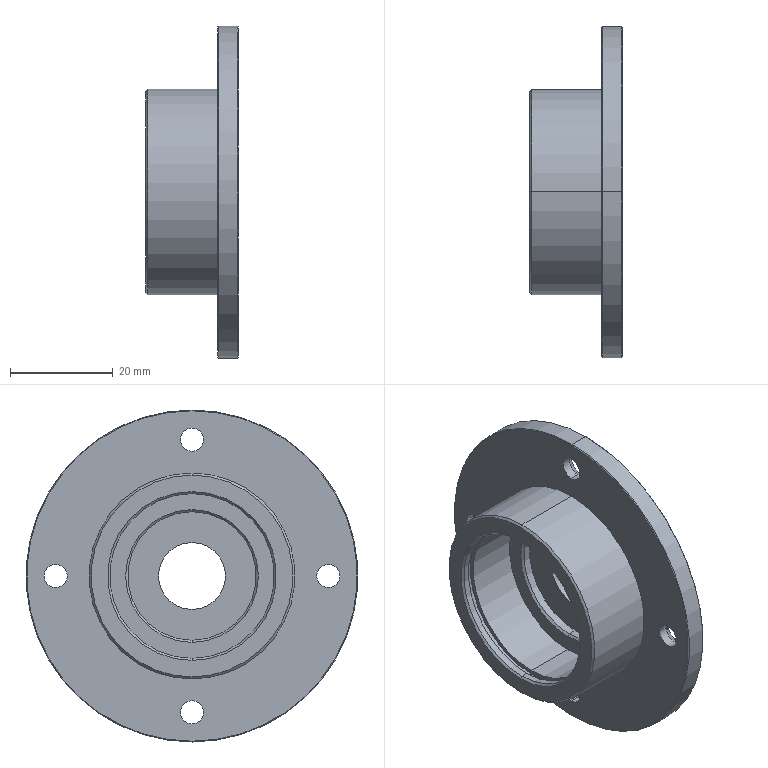Part | SolidWorks | features CirPattern 2, ICE 2, Chamfer 1, HoleWzd 1, RevCut 1, Revolution 1 | 1 solid | 47 faces | box 18 x 64.5 x 64.5 mm | volume 18239 mm3 | cylinder 22 | cone 18 | plane 7 | commonest cylinder face diameters 4.5 x8 32 x4 13 x2 25 x2 33.7 x2 40 x2
STEP:
#1=CARTESIAN_POINT('',(14.15,0.,32.25));
#2=VERTEX_POINT('',#1);
#3=CARTESIAN_POINT('',(14.15,0.,-32.25));
#4=VERTEX_POINT('',#3);
#5=CARTESIAN_POINT('',(14.15,0.,0.));
#6=DIRECTION('',(-1.,0.,0.));
#7=DIRECTION('',(0.,0.,-1.));
#8=AXIS2_PLACEMENT_3D('',#5,#6,#7);
#9=CIRCLE('',#8,32.25);
#10=EDGE_CURVE('',#2,#4,#9,.T.);
#11=ORIENTED_EDGE('',*,*,#10,.F.);
#12=CARTESIAN_POINT('',(17.85,0.,32.25));
#13=VERTEX_POINT('',#12);
#14=CARTESIAN_POINT('',(8.,0.,32.25));
#15=DIRECTION('',(1.,0.,0.));
#16=VECTOR('',#15,1000.);
#17=LINE('',#14,#16);
#18=EDGE_CURVE('',#2,#13,#17,.T.);
#19=ORIENTED_EDGE('',*,*,#18,.T.);
#20=CARTESIAN_POINT('',(17.85,0.,-32.25));
#21=VERTEX_POINT('',#20);
#22=CARTESIAN_POINT('',(17.85,0.,0.));
#23=DIRECTION('',(1.,0.,0.));
#24=DIRECTION('',(0.,0.,1.));
#25=AXIS2_PLACEMENT_3D('',#22,#23,#24);
#26=CIRCLE('',#25,32.25);
#27=EDGE_CURVE('',#21,#13,#26,.T.);
#28=ORIENTED_EDGE('',*,*,#27,.F.);
#29=CARTESIAN_POINT('',(8.,0.,-32.25));
#30=DIRECTION('',(1.,0.,0.));
#31=VECTOR('',#30,1000.);
#32=LINE('',#29,#31);
#33=EDGE_CURVE('',#4,#21,#32,.T.);
#34=ORIENTED_EDGE('',*,*,#33,.F.);
#35=EDGE_LOOP('',(#11,#19,#28,#34));
#36=FACE_OUTER_BOUND('',#35,.T.);
#37=CARTESIAN_POINT('',(8.,0.,0.));
#38=DIRECTION('',(1.,0.,0.));
#39=DIRECTION('',(0.,0.,-1.));
#40=AXIS2_PLACEMENT_3D('',#37,#38,#39);
#41=CYLINDRICAL_SURFACE('',#40,32.25);
#42=ADVANCED_FACE('',(#36),#41,.T.);
#43=CARTESIAN_POINT('',(18.,0.,-6.5));
#44=VERTEX_POINT('',#43);
#45=CARTESIAN_POINT('',(18.,0.,6.5));
#46=VERTEX_POINT('',#45);
#47=CARTESIAN_POINT('',(18.,0.,0.));
#48=DIRECTION('',(-1.,0.,0.));
#49=DIRECTION('',(0.,0.,1.));
#50=AXIS2_PLACEMENT_3D('',#47,#48,#49);
#51=CIRCLE('',#50,6.5);
#52=EDGE_CURVE('',#44,#46,#51,.T.);
#53=ORIENTED_EDGE('',*,*,#52,.F.);
#54=CARTESIAN_POINT('',(15.,0.,-6.5));
#55=VERTEX_POINT('',#54);
#56=CARTESIAN_POINT('',(25.,0.,-6.5));
#57=DIRECTION('',(-1.,0.,0.));
#58=VECTOR('',#57,1000.);
#59=LINE('',#56,#58);
#60=EDGE_CURVE('',#44,#55,#59,.T.);
#61=ORIENTED_EDGE('',*,*,#60,.T.);
#62=CARTESIAN_POINT('',(15.,0.,6.5));
#63=VERTEX_POINT('',#62);
#64=CARTESIAN_POINT('',(15.,0.,0.));
#65=DIRECTION('',(-1.,0.,0.));
#66=DIRECTION('',(0.,0.,1.));
#67=AXIS2_PLACEMENT_3D('',#64,#65,#66);
#68=CIRCLE('',#67,6.5);
#69=EDGE_CURVE('',#55,#63,#68,.T.);
#70=ORIENTED_EDGE('',*,*,#69,.T.);
#71=CARTESIAN_POINT('',(25.,0.,6.5));
#72=DIRECTION('',(-1.,0.,0.));
#73=VECTOR('',#72,1000.);
#74=LINE('',#71,#73);
#75=EDGE_CURVE('',#46,#63,#74,.T.);
#76=ORIENTED_EDGE('',*,*,#75,.F.);
#77=EDGE_LOOP('',(#53,#61,#70,#76));
#78=FACE_OUTER_BOUND('',#77,.T.);
#79=CARTESIAN_POINT('',(25.,0.,0.));
#80=DIRECTION('',(-1.,0.,0.));
#81=DIRECTION('',(0.,0.,1.));
#82=AXIS2_PLACEMENT_3D('',#79,#80,#81);
#83=CYLINDRICAL_SURFACE('',#82,6.5);
#84=ADVANCED_FACE('',(#78),#83,.F.);
#85=CARTESIAN_POINT('',(0.,0.,19.6));
#86=VERTEX_POINT('',#85);
#87=CARTESIAN_POINT('',(0.,0.,-19.6));
#88=VERTEX_POINT('',#87);
#89=CARTESIAN_POINT('',(0.,0.,0.));
#90=DIRECTION('',(-1.,0.,0.));
#91=DIRECTION('',(0.,0.,-1.));
#92=AXIS2_PLACEMENT_3D('',#89,#90,#91);
#93=CIRCLE('',#92,19.6);
#94=EDGE_CURVE('',#86,#88,#93,.T.);
#95=ORIENTED_EDGE('',*,*,#94,.F.);
#96=CARTESIAN_POINT('',(0.4,0.,20.));
#97=VERTEX_POINT('',#96);
#98=CARTESIAN_POINT('',(0.,0.,19.6));
#99=DIRECTION('',(0.7071,0.,0.7071));
#100=VECTOR('',#99,1000.);
#101=LINE('',#98,#100);
#102=EDGE_CURVE('',#86,#97,#101,.T.);
#103=ORIENTED_EDGE('',*,*,#102,.T.);
#104=CARTESIAN_POINT('',(0.4,0.,-20.));
#105=VERTEX_POINT('',#104);
#106=CARTESIAN_POINT('',(0.4,0.,0.));
#107=DIRECTION('',(1.,0.,0.));
#108=DIRECTION('',(0.,0.,-1.));
#109=AXIS2_PLACEMENT_3D('',#106,#107,#108);
#110=CIRCLE('',#109,20.);
#111=EDGE_CURVE('',#105,#97,#110,.T.);
#112=ORIENTED_EDGE('',*,*,#111,.F.);
#113=CARTESIAN_POINT('',(0.,0.,-19.6));
#114=DIRECTION('',(0.7071,0.,-0.7071));
#115=VECTOR('',#114,1000.);
#116=LINE('',#113,#115);
#117=EDGE_CURVE('',#88,#105,#116,.T.);
#118=ORIENTED_EDGE('',*,*,#117,.F.);
#119=EDGE_LOOP('',(#95,#103,#112,#118));
#120=FACE_OUTER_BOUND('',#119,.T.);
#121=CARTESIAN_POINT('',(0.,0.,0.));
#122=DIRECTION('',(1.,0.,0.));
#123=DIRECTION('',(0.,0.,-1.));
#124=AXIS2_PLACEMENT_3D('',#121,#122,#123);
#125=CONICAL_SURFACE('',#124,19.6,0.7854);
#126=ADVANCED_FACE('',(#120),#125,.T.);
#127=CARTESIAN_POINT('',(0.4,0.,-16.));
#128=VERTEX_POINT('',#127);
#129=CARTESIAN_POINT('',(0.4,0.,16.));
#130=VERTEX_POINT('',#129);
#131=CARTESIAN_POINT('',(0.4,0.,0.));
#132=DIRECTION('',(-1.,0.,0.));
#133=DIRECTION('',(0.,0.,-1.));
#134=AXIS2_PLACEMENT_3D('',#131,#132,#133);
#135=CIRCLE('',#134,16.);
#136=EDGE_CURVE('',#128,#130,#135,.T.);
#137=ORIENTED_EDGE('',*,*,#136,.F.);
#138=CARTESIAN_POINT('',(0.,0.,-16.4));
#139=VERTEX_POINT('',#138);
#140=CARTESIAN_POINT('',(0.4,0.,-16.));
#141=DIRECTION('',(-0.7071,0.,-0.7071));
#142=VECTOR('',#141,1000.);
#143=LINE('',#140,#142);
#144=EDGE_CURVE('',#128,#139,#143,.T.);
#145=ORIENTED_EDGE('',*,*,#144,.T.);
#146=CARTESIAN_POINT('',(0.,0.,16.4));
#147=VERTEX_POINT('',#146);
#148=CARTESIAN_POINT('',(0.,0.,0.));
#149=DIRECTION('',(1.,0.,0.));
#150=DIRECTION('',(0.,0.,-1.));
#151=AXIS2_PLACEMENT_3D('',#148,#149,#150);
#152=CIRCLE('',#151,16.4);
#153=EDGE_CURVE('',#147,#139,#152,.T.);
#154=ORIENTED_EDGE('',*,*,#153,.F.);
#155=CARTESIAN_POINT('',(0.4,0.,16.));
#156=DIRECTION('',(-0.7071,0.,0.7071));
#157=VECTOR('',#156,1000.);
#158=LINE('',#155,#157);
#159=EDGE_CURVE('',#130,#147,#158,.T.);
#160=ORIENTED_EDGE('',*,*,#159,.F.);
#161=EDGE_LOOP('',(#137,#145,#154,#160));
#162=FACE_OUTER_BOUND('',#161,.T.);
#163=CARTESIAN_POINT('',(0.4,0.,0.));
#164=DIRECTION('',(-1.,0.,0.));
#165=DIRECTION('',(0.,0.,1.));
#166=AXIS2_PLACEMENT_3D('',#163,#164,#165);
#167=CONICAL_SURFACE('',#166,16.,0.7854);
#168=ADVANCED_FACE('',(#162),#167,.F.);
#169=CARTESIAN_POINT('',(13.4,0.,-12.5));
#170=VERTEX_POINT('',#169);
#171=CARTESIAN_POINT('',(13.4,0.,12.5));
#172=VERTEX_POINT('',#171);
#173=CARTESIAN_POINT('',(13.4,0.,0.));
#174=DIRECTION('',(-1.,0.,0.));
#175=DIRECTION('',(0.,0.,-1.));
#176=AXIS2_PLACEMENT_3D('',#173,#174,#175);
#177=CIRCLE('',#176,12.5);
#178=EDGE_CURVE('',#170,#172,#177,.T.);
#179=ORIENTED_EDGE('',*,*,#178,.F.);
#180=CARTESIAN_POINT('',(13.,0.,-12.9));
#181=VERTEX_POINT('',#180);
#182=CARTESIAN_POINT('',(13.4,0.,-12.5));
#183=DIRECTION('',(-0.7071,0.,-0.7071));
#184=VECTOR('',#183,1000.);
#185=LINE('',#182,#184);
#186=EDGE_CURVE('',#170,#181,#185,.T.);
#187=ORIENTED_EDGE('',*,*,#186,.T.);
#188=CARTESIAN_POINT('',(13.,0.,12.9));
#189=VERTEX_POINT('',#188);
#190=CARTESIAN_POINT('',(13.,0.,0.));
#191=DIRECTION('',(1.,0.,0.));
#192=DIRECTION('',(0.,0.,-1.));
#193=AXIS2_PLACEMENT_3D('',#190,#191,#192);
#194=CIRCLE('',#193,12.9);
#195=EDGE_CURVE('',#189,#181,#194,.T.);
#196=ORIENTED_EDGE('',*,*,#195,.F.);
#197=CARTESIAN_POINT('',(13.4,0.,12.5));
#198=DIRECTION('',(-0.7071,0.,0.7071));
#199=VECTOR('',#198,1000.);
#200=LINE('',#197,#199);
#201=EDGE_CURVE('',#172,#189,#200,.T.);
#202=ORIENTED_EDGE('',*,*,#201,.F.);
#203=EDGE_LOOP('',(#179,#187,#196,#202));
#204=FACE_OUTER_BOUND('',#203,.T.);
#205=CARTESIAN_POINT('',(13.4,0.,0.));
#206=DIRECTION('',(-1.,0.,0.));
#207=DIRECTION('',(0.,0.,1.));
#208=AXIS2_PLACEMENT_3D('',#205,#206,#207);
#209=CONICAL_SURFACE('',#208,12.5,0.7854);
#210=ADVANCED_FACE('',(#204),#209,.F.);
#211=CARTESIAN_POINT('',(15.75,28.75,0.));
#212=VERTEX_POINT('',#211);
#213=CARTESIAN_POINT('',(15.75,24.25,0.));
#214=VERTEX_POINT('',#213);
#215=CARTESIAN_POINT('',(15.75,26.5,0.));
#216=DIRECTION('',(-1.,0.,0.));
#217=DIRECTION('',(0.,-1.,0.));
#218=AXIS2_PLACEMENT_3D('',#215,#216,#217);
#219=CIRCLE('',#218,2.25);
#220=EDGE_CURVE('',#212,#214,#219,.T.);
#221=ORIENTED_EDGE('',*,*,#220,.F.);
#222=CARTESIAN_POINT('',(14.,28.75,0.));
#223=VERTEX_POINT('',#222);
#224=CARTESIAN_POINT('',(14.,28.75,0.));
#225=DIRECTION('',(-1.,0.,0.));
#226=VECTOR('',#225,1000.);
#227=LINE('',#224,#226);
#228=EDGE_CURVE('',#212,#223,#227,.T.);
#229=ORIENTED_EDGE('',*,*,#228,.T.);
#230=CARTESIAN_POINT('',(14.,24.25,0.));
#231=VERTEX_POINT('',#230);
#232=CARTESIAN_POINT('',(14.,26.5,0.));
#233=DIRECTION('',(-1.,0.,0.));
#234=DIRECTION('',(0.,-1.,0.));
#235=AXIS2_PLACEMENT_3D('',#232,#233,#234);
#236=CIRCLE('',#235,2.25);
#237=EDGE_CURVE('',#223,#231,#236,.T.);
#238=ORIENTED_EDGE('',*,*,#237,.T.);
#239=CARTESIAN_POINT('',(14.,24.25,0.));
#240=DIRECTION('',(-1.,0.,0.));
#241=VECTOR('',#240,1000.);
#242=LINE('',#239,#241);
#243=EDGE_CURVE('',#214,#231,#242,.T.);
#244=ORIENTED_EDGE('',*,*,#243,.F.);
#245=EDGE_LOOP('',(#221,#229,#238,#244));
#246=FACE_OUTER_BOUND('',#245,.T.);
#247=CARTESIAN_POINT('',(14.,26.5,0.));
#248=DIRECTION('',(-1.,0.,0.));
#249=DIRECTION('',(0.,-1.,0.));
#250=AXIS2_PLACEMENT_3D('',#247,#248,#249);
#251=CYLINDRICAL_SURFACE('',#250,2.25);
#252=ADVANCED_FACE('',(#246),#251,.F.);
#253=ORIENTED_EDGE('',*,*,#220,.T.);
#254=CARTESIAN_POINT('',(18.,22.,0.));
#255=VERTEX_POINT('',#254);
#256=CARTESIAN_POINT('',(18.,22.,0.));
#257=DIRECTION('',(0.7071,-0.7071,0.));
#258=VECTOR('',#257,1000.);
#259=LINE('',#256,#258);
#260=EDGE_CURVE('',#214,#255,#259,.T.);
#261=ORIENTED_EDGE('',*,*,#260,.T.);
#262=CARTESIAN_POINT('',(18.,31.,0.));
#263=VERTEX_POINT('',#262);
#264=CARTESIAN_POINT('',(18.,26.5,0.));
#265=DIRECTION('',(-1.,0.,0.));
#266=DIRECTION('',(0.,-1.,0.));
#267=AXIS2_PLACEMENT_3D('',#264,#265,#266);
#268=CIRCLE('',#267,4.5);
#269=EDGE_CURVE('',#263,#255,#268,.T.);
#270=ORIENTED_EDGE('',*,*,#269,.F.);
#271=CARTESIAN_POINT('',(18.,31.,0.));
#272=DIRECTION('',(0.7071,0.7071,0.));
#273=VECTOR('',#272,1000.);
#274=LINE('',#271,#273);
#275=EDGE_CURVE('',#212,#263,#274,.T.);
#276=ORIENTED_EDGE('',*,*,#275,.F.);
#277=EDGE_LOOP('',(#253,#261,#270,#276));
#278=FACE_OUTER_BOUND('',#277,.T.);
#279=CARTESIAN_POINT('',(18.,26.5,0.));
#280=DIRECTION('',(1.,0.,0.));
#281=DIRECTION('',(0.,1.,0.));
#282=AXIS2_PLACEMENT_3D('',#279,#280,#281);
#283=CONICAL_SURFACE('',#282,4.5,0.7854);
#284=ADVANCED_FACE('',(#278),#283,.F.);
#285=CARTESIAN_POINT('',(15.75,0.,28.75));
#286=VERTEX_POINT('',#285);
#287=CARTESIAN_POINT('',(15.75,0.,24.25));
#288=VERTEX_POINT('',#287);
#289=CARTESIAN_POINT('',(15.75,0.,26.5));
#290=DIRECTION('',(-1.,0.,0.));
#291=DIRECTION('',(0.,0.,-1.));
#292=AXIS2_PLACEMENT_3D('',#289,#290,#291);
#293=CIRCLE('',#292,2.25);
#294=EDGE_CURVE('',#286,#288,#293,.T.);
#295=ORIENTED_EDGE('',*,*,#294,.F.);
#296=CARTESIAN_POINT('',(14.,0.,28.75));
#297=VERTEX_POINT('',#296);
#298=CARTESIAN_POINT('',(14.,0.,28.75));
#299=DIRECTION('',(-1.,0.,0.));
#300=VECTOR('',#299,1000.);
#301=LINE('',#298,#300);
#302=EDGE_CURVE('',#286,#297,#301,.T.);
#303=ORIENTED_EDGE('',*,*,#302,.T.);
#304=CARTESIAN_POINT('',(14.,0.,24.25));
#305=VERTEX_POINT('',#304);
#306=CARTESIAN_POINT('',(14.,0.,26.5));
#307=DIRECTION('',(-1.,0.,0.));
#308=DIRECTION('',(0.,0.,-1.));
#309=AXIS2_PLACEMENT_3D('',#306,#307,#308);
#310=CIRCLE('',#309,2.25);
#311=EDGE_CURVE('',#297,#305,#310,.T.);
#312=ORIENTED_EDGE('',*,*,#311,.T.);
#313=CARTESIAN_POINT('',(14.,0.,24.25));
#314=DIRECTION('',(-1.,0.,0.));
#315=VECTOR('',#314,1000.);
#316=LINE('',#313,#315);
#317=EDGE_CURVE('',#288,#305,#316,.T.);
#318=ORIENTED_EDGE('',*,*,#317,.F.);
#319=EDGE_LOOP('',(#295,#303,#312,#318));
#320=FACE_OUTER_BOUND('',#319,.T.);
#321=CARTESIAN_POINT('',(14.,0.,26.5));
#322=DIRECTION('',(-1.,0.,0.));
#323=DIRECTION('',(0.,0.,-1.));
#324=AXIS2_PLACEMENT_3D('',#321,#322,#323);
#325=CYLINDRICAL_SURFACE('',#324,2.25);
#326=ADVANCED_FACE('',(#320),#325,.F.);
#327=ORIENTED_EDGE('',*,*,#294,.T.);
#328=CARTESIAN_POINT('',(18.,0.,22.));
#329=VERTEX_POINT('',#328);
#330=CARTESIAN_POINT('',(18.,0.,22.));
#331=DIRECTION('',(0.7071,0.,-0.7071));
#332=VECTOR('',#331,1000.);
#333=LINE('',#330,#332);
#334=EDGE_CURVE('',#288,#329,#333,.T.);
#335=ORIENTED_EDGE('',*,*,#334,.T.);
#336=CARTESIAN_POINT('',(18.,0.,31.));
#337=VERTEX_POINT('',#336);
#338=CARTESIAN_POINT('',(18.,0.,26.5));
#339=DIRECTION('',(-1.,0.,0.));
#340=DIRECTION('',(0.,0.,-1.));
#341=AXIS2_PLACEMENT_3D('',#338,#339,#340);
#342=CIRCLE('',#341,4.5);
#343=EDGE_CURVE('',#337,#329,#342,.T.);
#344=ORIENTED_EDGE('',*,*,#343,.F.);
#345=CARTESIAN_POINT('',(18.,0.,31.));
#346=DIRECTION('',(0.7071,0.,0.7071));
#347=VECTOR('',#346,1000.);
#348=LINE('',#345,#347);
#349=EDGE_CURVE('',#286,#337,#348,.T.);
#350=ORIENTED_EDGE('',*,*,#349,.F.);
#351=EDGE_LOOP('',(#327,#335,#344,#350));
#352=FACE_OUTER_BOUND('',#351,.T.);
#353=CARTESIAN_POINT('',(18.,0.,26.5));
#354=DIRECTION('',(1.,0.,0.));
#355=DIRECTION('',(0.,0.,1.));
#356=AXIS2_PLACEMENT_3D('',#353,#354,#355);
#357=CONICAL_SURFACE('',#356,4.5,0.7854);
#358=ADVANCED_FACE('',(#352),#357,.F.);
#359=CARTESIAN_POINT('',(15.75,-28.75,0.));
#360=VERTEX_POINT('',#359);
#361=CARTESIAN_POINT('',(15.75,-24.25,0.));
#362=VERTEX_POINT('',#361);
#363=CARTESIAN_POINT('',(15.75,-26.5,0.));
#364=DIRECTION('',(-1.,0.,0.));
#365=DIRECTION('',(0.,1.,0.));
#366=AXIS2_PLACEMENT_3D('',#363,#364,#365);
#367=CIRCLE('',#366,2.25);
#368=EDGE_CURVE('',#360,#362,#367,.T.);
#369=ORIENTED_EDGE('',*,*,#368,.F.);
#370=CARTESIAN_POINT('',(14.,-28.75,0.));
#371=VERTEX_POINT('',#370);
#372=CARTESIAN_POINT('',(14.,-28.75,0.));
#373=DIRECTION('',(-1.,0.,0.));
#374=VECTOR('',#373,1000.);
#375=LINE('',#372,#374);
#376=EDGE_CURVE('',#360,#371,#375,.T.);
#377=ORIENTED_EDGE('',*,*,#376,.T.);
#378=CARTESIAN_POINT('',(14.,-24.25,0.));
#379=VERTEX_POINT('',#378);
#380=CARTESIAN_POINT('',(14.,-26.5,0.));
#381=DIRECTION('',(-1.,0.,0.));
#382=DIRECTION('',(0.,1.,0.));
#383=AXIS2_PLACEMENT_3D('',#380,#381,#382);
#384=CIRCLE('',#383,2.25);
#385=EDGE_CURVE('',#371,#379,#384,.T.);
#386=ORIENTED_EDGE('',*,*,#385,.T.);
#387=CARTESIAN_POINT('',(14.,-24.25,0.));
#388=DIRECTION('',(-1.,0.,0.));
#389=VECTOR('',#388,1000.);
#390=LINE('',#387,#389);
#391=EDGE_CURVE('',#362,#379,#390,.T.);
#392=ORIENTED_EDGE('',*,*,#391,.F.);
#393=EDGE_LOOP('',(#369,#377,#386,#392));
#394=FACE_OUTER_BOUND('',#393,.T.);
#395=CARTESIAN_POINT('',(14.,-26.5,0.));
#396=DIRECTION('',(-1.,0.,0.));
#397=DIRECTION('',(0.,1.,0.));
#398=AXIS2_PLACEMENT_3D('',#395,#396,#397);
#399=CYLINDRICAL_SURFACE('',#398,2.25);
#400=ADVANCED_FACE('',(#394),#399,.F.);
#401=ORIENTED_EDGE('',*,*,#368,.T.);
#402=CARTESIAN_POINT('',(18.,-22.,0.));
#403=VERTEX_POINT('',#402);
#404=CARTESIAN_POINT('',(18.,-22.,0.));
#405=DIRECTION('',(0.7071,0.7071,0.));
#406=VECTOR('',#405,1000.);
#407=LINE('',#404,#406);
#408=EDGE_CURVE('',#362,#403,#407,.T.);
#409=ORIENTED_EDGE('',*,*,#408,.T.);
#410=CARTESIAN_POINT('',(18.,-31.,0.));
#411=VERTEX_POINT('',#410);
#412=CARTESIAN_POINT('',(18.,-26.5,0.));
#413=DIRECTION('',(-1.,0.,0.));
#414=DIRECTION('',(0.,1.,0.));
#415=AXIS2_PLACEMENT_3D('',#412,#413,#414);
#416=CIRCLE('',#415,4.5);
#417=EDGE_CURVE('',#411,#403,#416,.T.);
#418=ORIENTED_EDGE('',*,*,#417,.F.);
#419=CARTESIAN_POINT('',(18.,-31.,0.));
#420=DIRECTION('',(0.7071,-0.7071,0.));
#421=VECTOR('',#420,1000.);
#422=LINE('',#419,#421);
#423=EDGE_CURVE('',#360,#411,#422,.T.);
#424=ORIENTED_EDGE('',*,*,#423,.F.);
#425=EDGE_LOOP('',(#401,#409,#418,#424));
#426=FACE_OUTER_BOUND('',#425,.T.);
#427=CARTESIAN_POINT('',(18.,-26.5,0.));
#428=DIRECTION('',(1.,0.,0.));
#429=DIRECTION('',(0.,-1.,0.));
#430=AXIS2_PLACEMENT_3D('',#427,#428,#429);
#431=CONICAL_SURFACE('',#430,4.5,0.7854);
#432=ADVANCED_FACE('',(#426),#431,.F.);
#433=CARTESIAN_POINT('',(15.75,0.,-28.75));
#434=VERTEX_POINT('',#433);
#435=CARTESIAN_POINT('',(15.75,0.,-24.25));
#436=VERTEX_POINT('',#435);
#437=CARTESIAN_POINT('',(15.75,0.,-26.5));
#438=DIRECTION('',(-1.,0.,0.));
#439=DIRECTION('',(0.,0.,1.));
#440=AXIS2_PLACEMENT_3D('',#437,#438,#439);
#441=CIRCLE('',#440,2.25);
#442=EDGE_CURVE('',#434,#436,#441,.T.);
#443=ORIENTED_EDGE('',*,*,#442,.F.);
#444=CARTESIAN_POINT('',(14.,0.,-28.75));
#445=VERTEX_POINT('',#444);
#446=CARTESIAN_POINT('',(14.,0.,-28.75));
#447=DIRECTION('',(-1.,0.,0.));
#448=VECTOR('',#447,1000.);
#449=LINE('',#446,#448);
#450=EDGE_CURVE('',#434,#445,#449,.T.);
#451=ORIENTED_EDGE('',*,*,#450,.T.);
#452=CARTESIAN_POINT('',(14.,0.,-24.25));
#453=VERTEX_POINT('',#452);
#454=CARTESIAN_POINT('',(14.,0.,-26.5));
#455=DIRECTION('',(-1.,0.,0.));
#456=DIRECTION('',(0.,0.,1.));
#457=AXIS2_PLACEMENT_3D('',#454,#455,#456);
#458=CIRCLE('',#457,2.25);
#459=EDGE_CURVE('',#445,#453,#458,.T.);
#460=ORIENTED_EDGE('',*,*,#459,.T.);
#461=CARTESIAN_POINT('',(14.,0.,-24.25));
#462=DIRECTION('',(-1.,0.,0.));
#463=VECTOR('',#462,1000.);
#464=LINE('',#461,#463);
#465=EDGE_CURVE('',#436,#453,#464,.T.);
#466=ORIENTED_EDGE('',*,*,#465,.F.);
#467=EDGE_LOOP('',(#443,#451,#460,#466));
#468=FACE_OUTER_BOUND('',#467,.T.);
#469=CARTESIAN_POINT('',(14.,0.,-26.5));
#470=DIRECTION('',(-1.,0.,0.));
#471=DIRECTION('',(0.,0.,1.));
#472=AXIS2_PLACEMENT_3D('',#469,#470,#471);
#473=CYLINDRICAL_SURFACE('',#472,2.25);
#474=ADVANCED_FACE('',(#468),#473,.F.);
#475=ORIENTED_EDGE('',*,*,#442,.T.);
#476=CARTESIAN_POINT('',(18.,0.,-22.));
#477=VERTEX_POINT('',#476);
#478=CARTESIAN_POINT('',(18.,0.,-22.));
#479=DIRECTION('',(0.7071,0.,0.7071));
#480=VECTOR('',#479,1000.);
#481=LINE('',#478,#480);
#482=EDGE_CURVE('',#436,#477,#481,.T.);
#483=ORIENTED_EDGE('',*,*,#482,.T.);
#484=CARTESIAN_POINT('',(18.,0.,-31.));
#485=VERTEX_POINT('',#484);
#486=CARTESIAN_POINT('',(18.,0.,-26.5));
#487=DIRECTION('',(-1.,0.,0.));
#488=DIRECTION('',(0.,0.,1.));
#489=AXIS2_PLACEMENT_3D('',#486,#487,#488);
#490=CIRCLE('',#489,4.5);
#491=EDGE_CURVE('',#485,#477,#490,.T.);
#492=ORIENTED_EDGE('',*,*,#491,.F.);
#493=CARTESIAN_POINT('',(18.,0.,-31.));
#494=DIRECTION('',(0.7071,0.,-0.7071));
#495=VECTOR('',#494,1000.);
#496=LINE('',#493,#495);
#497=EDGE_CURVE('',#434,#485,#496,.T.);
#498=ORIENTED_EDGE('',*,*,#497,.F.);
#499=EDGE_LOOP('',(#475,#483,#492,#498));
#500=FACE_OUTER_BOUND('',#499,.T.);
#501=CARTESIAN_POINT('',(18.,0.,-26.5));
#502=DIRECTION('',(1.,0.,0.));
#503=DIRECTION('',(0.,0.,-1.));
#504=AXIS2_PLACEMENT_3D('',#501,#502,#503);
#505=CONICAL_SURFACE('',#504,4.5,0.7854);
#506=ADVANCED_FACE('',(#500),#505,.F.);
#507=CARTESIAN_POINT('',(14.,0.,20.));
#508=VERTEX_POINT('',#507);
#509=CARTESIAN_POINT('',(14.,0.,-20.));
#510=VERTEX_POINT('',#509);
#511=CARTESIAN_POINT('',(14.,0.,0.));
#512=DIRECTION('',(-1.,0.,0.));
#513=DIRECTION('',(0.,0.,1.));
#514=AXIS2_PLACEMENT_3D('',#511,#512,#513);
#515=CIRCLE('',#514,20.);
#516=EDGE_CURVE('',#508,#510,#515,.T.);
#517=ORIENTED_EDGE('',*,*,#516,.T.);
#518=CARTESIAN_POINT('',(15.,0.,-20.));
#519=DIRECTION('',(-1.,0.,0.));
#520=VECTOR('',#519,1000.);
#521=LINE('',#518,#520);
#522=EDGE_CURVE('',#510,#105,#521,.T.);
#523=ORIENTED_EDGE('',*,*,#522,.T.);
#524=ORIENTED_EDGE('',*,*,#111,.T.);
#525=CARTESIAN_POINT('',(15.,0.,20.));
#526=DIRECTION('',(-1.,0.,0.));
#527=VECTOR('',#526,1000.);
#528=LINE('',#525,#527);
#529=EDGE_CURVE('',#508,#97,#528,.T.);
#530=ORIENTED_EDGE('',*,*,#529,.F.);
#531=EDGE_LOOP('',(#517,#523,#524,#530));
#532=FACE_OUTER_BOUND('',#531,.T.);
#533=CARTESIAN_POINT('',(15.,0.,0.));
#534=DIRECTION('',(-1.,0.,0.));
#535=DIRECTION('',(0.,0.,1.));
#536=AXIS2_PLACEMENT_3D('',#533,#534,#535);
#537=CYLINDRICAL_SURFACE('',#536,20.);
#538=ADVANCED_FACE('',(#532),#537,.T.);
#539=CARTESIAN_POINT('',(15.,0.,-12.5));
#540=VERTEX_POINT('',#539);
#541=CARTESIAN_POINT('',(15.,0.,12.5));
#542=VERTEX_POINT('',#541);
#543=CARTESIAN_POINT('',(15.,0.,0.));
#544=DIRECTION('',(-1.,0.,0.));
#545=DIRECTION('',(0.,0.,1.));
#546=AXIS2_PLACEMENT_3D('',#543,#544,#545);
#547=CIRCLE('',#546,12.5);
#548=EDGE_CURVE('',#540,#542,#547,.T.);
#549=ORIENTED_EDGE('',*,*,#548,.F.);
#550=CARTESIAN_POINT('',(15.,0.,-12.5));
#551=DIRECTION('',(-1.,0.,0.));
#552=VECTOR('',#551,1000.);
#553=LINE('',#550,#552);
#554=EDGE_CURVE('',#540,#170,#553,.T.);
#555=ORIENTED_EDGE('',*,*,#554,.T.);
#556=ORIENTED_EDGE('',*,*,#178,.T.);
#557=CARTESIAN_POINT('',(15.,0.,12.5));
#558=DIRECTION('',(-1.,0.,0.));
#559=VECTOR('',#558,1000.);
#560=LINE('',#557,#559);
#561=EDGE_CURVE('',#542,#172,#560,.T.);
#562=ORIENTED_EDGE('',*,*,#561,.F.);
#563=EDGE_LOOP('',(#549,#555,#556,#562));
#564=FACE_OUTER_BOUND('',#563,.T.);
#565=CARTESIAN_POINT('',(15.,0.,0.));
#566=DIRECTION('',(-1.,0.,0.));
#567=DIRECTION('',(0.,0.,1.));
#568=AXIS2_PLACEMENT_3D('',#565,#566,#567);
#569=CYLINDRICAL_SURFACE('',#568,12.5);
#570=ADVANCED_FACE('',(#564),#569,.F.);
#571=CARTESIAN_POINT('',(13.,0.,-16.));
#572=VERTEX_POINT('',#571);
#573=CARTESIAN_POINT('',(13.,0.,16.));
#574=VERTEX_POINT('',#573);
#575=CARTESIAN_POINT('',(13.,0.,0.));
#576=DIRECTION('',(-1.,0.,0.));
#577=DIRECTION('',(0.,0.,1.));
#578=AXIS2_PLACEMENT_3D('',#575,#576,#577);
#579=CIRCLE('',#578,16.);
#580=EDGE_CURVE('',#572,#574,#579,.T.);
#581=ORIENTED_EDGE('',*,*,#580,.F.);
#582=CARTESIAN_POINT('',(2.995,0.,-16.));
#583=VERTEX_POINT('',#582);
#584=CARTESIAN_POINT('',(15.,0.,-16.));
#585=DIRECTION('',(-1.,0.,0.));
#586=VECTOR('',#585,1000.);
#587=LINE('',#584,#586);
#588=EDGE_CURVE('',#572,#583,#587,.T.);
#589=ORIENTED_EDGE('',*,*,#588,.T.);
#590=CARTESIAN_POINT('',(2.995,0.,16.));
#591=VERTEX_POINT('',#590);
#592=CARTESIAN_POINT('',(2.995,0.,0.));
#593=DIRECTION('',(-1.,0.,0.));
#594=DIRECTION('',(0.,0.,1.));
#595=AXIS2_PLACEMENT_3D('',#592,#593,#594);
#596=CIRCLE('',#595,16.);
#597=EDGE_CURVE('',#583,#591,#596,.T.);
#598=ORIENTED_EDGE('',*,*,#597,.T.);
#599=CARTESIAN_POINT('',(15.,0.,16.));
#600=DIRECTION('',(-1.,0.,0.));
#601=VECTOR('',#600,1000.);
#602=LINE('',#599,#601);
#603=EDGE_CURVE('',#574,#591,#602,.T.);
#604=ORIENTED_EDGE('',*,*,#603,.F.);
#605=EDGE_LOOP('',(#581,#589,#598,#604));
#606=FACE_OUTER_BOUND('',#605,.T.);
#607=CARTESIAN_POINT('',(15.,0.,0.));
#608=DIRECTION('',(-1.,0.,0.));
#609=DIRECTION('',(0.,0.,1.));
#610=AXIS2_PLACEMENT_3D('',#607,#608,#609);
#611=CYLINDRICAL_SURFACE('',#610,16.);
#612=ADVANCED_FACE('',(#606),#611,.F.);
#613=CARTESIAN_POINT('',(2.995,0.,-16.85));
#614=VERTEX_POINT('',#613);
#615=CARTESIAN_POINT('',(2.995,0.,16.85));
#616=VERTEX_POINT('',#615);
#617=CARTESIAN_POINT('',(2.995,0.,0.));
#618=DIRECTION('',(-1.,0.,0.));
#619=DIRECTION('',(0.,0.,1.));
#620=AXIS2_PLACEMENT_3D('',#617,#618,#619);
#621=CIRCLE('',#620,16.85);
#622=EDGE_CURVE('',#614,#616,#621,.T.);
#623=ORIENTED_EDGE('',*,*,#622,.F.);
#624=CARTESIAN_POINT('',(1.695,0.,-16.85));
#625=VERTEX_POINT('',#624);
#626=CARTESIAN_POINT('',(15.,0.,-16.85));
#627=DIRECTION('',(-1.,0.,0.));
#628=VECTOR('',#627,1000.);
#629=LINE('',#626,#628);
#630=EDGE_CURVE('',#614,#625,#629,.T.);
#631=ORIENTED_EDGE('',*,*,#630,.T.);
#632=CARTESIAN_POINT('',(1.695,0.,16.85));
#633=VERTEX_POINT('',#632);
#634=CARTESIAN_POINT('',(1.695,0.,0.));
#635=DIRECTION('',(-1.,0.,0.));
#636=DIRECTION('',(0.,0.,1.));
#637=AXIS2_PLACEMENT_3D('',#634,#635,#636);
#638=CIRCLE('',#637,16.85);
#639=EDGE_CURVE('',#625,#633,#638,.T.);
#640=ORIENTED_EDGE('',*,*,#639,.T.);
#641=CARTESIAN_POINT('',(15.,0.,16.85));
#642=DIRECTION('',(-1.,0.,0.));
#643=VECTOR('',#642,1000.);
#644=LINE('',#641,#643);
#645=EDGE_CURVE('',#616,#633,#644,.T.);
#646=ORIENTED_EDGE('',*,*,#645,.F.);
#647=EDGE_LOOP('',(#623,#631,#640,#646));
#648=FACE_OUTER_BOUND('',#647,.T.);
#649=CARTESIAN_POINT('',(15.,0.,0.));
#650=DIRECTION('',(-1.,0.,0.));
#651=DIRECTION('',(0.,0.,1.));
#652=AXIS2_PLACEMENT_3D('',#649,#650,#651);
#653=CYLINDRICAL_SURFACE('',#652,16.85);
#654=ADVANCED_FACE('',(#648),#653,.F.);
#655=CARTESIAN_POINT('',(1.695,0.,-16.));
#656=VERTEX_POINT('',#655);
#657=CARTESIAN_POINT('',(1.695,0.,16.));
#658=VERTEX_POINT('',#657);
#659=CARTESIAN_POINT('',(1.695,0.,0.));
#660=DIRECTION('',(-1.,0.,0.));
#661=DIRECTION('',(0.,0.,1.));
#662=AXIS2_PLACEMENT_3D('',#659,#660,#661);
#663=CIRCLE('',#662,16.);
#664=EDGE_CURVE('',#656,#658,#663,.T.);
#665=ORIENTED_EDGE('',*,*,#664,.F.);
#666=CARTESIAN_POINT('',(15.,0.,-16.));
#667=DIRECTION('',(-1.,0.,0.));
#668=VECTOR('',#667,1000.);
#669=LINE('',#666,#668);
#670=EDGE_CURVE('',#656,#128,#669,.T.);
#671=ORIENTED_EDGE('',*,*,#670,.T.);
#672=ORIENTED_EDGE('',*,*,#136,.T.);
#673=CARTESIAN_POINT('',(15.,0.,16.));
#674=DIRECTION('',(-1.,0.,0.));
#675=VECTOR('',#674,1000.);
#676=LINE('',#673,#675);
#677=EDGE_CURVE('',#658,#130,#676,.T.);
#678=ORIENTED_EDGE('',*,*,#677,.F.);
#679=EDGE_LOOP('',(#665,#671,#672,#678));
#680=FACE_OUTER_BOUND('',#679,.T.);
#681=CARTESIAN_POINT('',(15.,0.,0.));
#682=DIRECTION('',(-1.,0.,0.));
#683=DIRECTION('',(0.,0.,1.));
#684=AXIS2_PLACEMENT_3D('',#681,#682,#683);
#685=CYLINDRICAL_SURFACE('',#684,16.);
#686=ADVANCED_FACE('',(#680),#685,.F.);
#687=CARTESIAN_POINT('',(14.,0.,32.1));
#688=VERTEX_POINT('',#687);
#689=CARTESIAN_POINT('',(14.,0.,-32.1));
#690=VERTEX_POINT('',#689);
#691=CARTESIAN_POINT('',(14.,0.,0.));
#692=DIRECTION('',(-1.,0.,0.));
#693=DIRECTION('',(0.,0.,-1.));
#694=AXIS2_PLACEMENT_3D('',#691,#692,#693);
#695=CIRCLE('',#694,32.1);
#696=EDGE_CURVE('',#688,#690,#695,.T.);
#697=ORIENTED_EDGE('',*,*,#696,.F.);
#698=CARTESIAN_POINT('',(14.,0.,32.1));
#699=DIRECTION('',(0.7071,0.,0.7071));
#700=VECTOR('',#699,1000.);
#701=LINE('',#698,#700);
#702=EDGE_CURVE('',#688,#2,#701,.T.);
#703=ORIENTED_EDGE('',*,*,#702,.T.);
#704=ORIENTED_EDGE('',*,*,#10,.T.);
#705=CARTESIAN_POINT('',(14.,0.,-32.1));
#706=DIRECTION('',(0.7071,0.,-0.7071));
#707=VECTOR('',#706,1000.);
#708=LINE('',#705,#707);
#709=EDGE_CURVE('',#690,#4,#708,.T.);
#710=ORIENTED_EDGE('',*,*,#709,.F.);
#711=EDGE_LOOP('',(#697,#703,#704,#710));
#712=FACE_OUTER_BOUND('',#711,.T.);
#713=CARTESIAN_POINT('',(14.,0.,0.));
#714=DIRECTION('',(1.,0.,0.));
#715=DIRECTION('',(0.,0.,-1.));
#716=AXIS2_PLACEMENT_3D('',#713,#714,#715);
#717=CONICAL_SURFACE('',#716,32.1,0.7854);
#718=ADVANCED_FACE('',(#712),#717,.T.);
#719=CARTESIAN_POINT('',(18.,0.,-32.1));
#720=VERTEX_POINT('',#719);
#721=CARTESIAN_POINT('',(18.,0.,32.1));
#722=VERTEX_POINT('',#721);
#723=CARTESIAN_POINT('',(18.,0.,0.));
#724=DIRECTION('',(1.,0.,0.));
#725=DIRECTION('',(0.,0.,1.));
#726=AXIS2_PLACEMENT_3D('',#723,#724,#725);
#727=CIRCLE('',#726,32.1);
#728=EDGE_CURVE('',#720,#722,#727,.T.);
#729=ORIENTED_EDGE('',*,*,#728,.F.);
#730=CARTESIAN_POINT('',(17.6,0.,-32.5));
#731=DIRECTION('',(-0.7071,0.,-0.7071));
#732=VECTOR('',#731,1000.);
#733=LINE('',#730,#732);
#734=EDGE_CURVE('',#720,#21,#733,.T.);
#735=ORIENTED_EDGE('',*,*,#734,.T.);
#736=ORIENTED_EDGE('',*,*,#27,.T.);
#737=CARTESIAN_POINT('',(17.6,0.,32.5));
#738=DIRECTION('',(-0.7071,0.,0.7071));
#739=VECTOR('',#738,1000.);
#740=LINE('',#737,#739);
#741=EDGE_CURVE('',#722,#13,#740,.T.);
#742=ORIENTED_EDGE('',*,*,#741,.F.);
#743=EDGE_LOOP('',(#729,#735,#736,#742));
#744=FACE_OUTER_BOUND('',#743,.T.);
#745=CARTESIAN_POINT('',(17.6,0.,0.));
#746=DIRECTION('',(-1.,0.,0.));
#747=DIRECTION('',(0.,0.,1.));
#748=AXIS2_PLACEMENT_3D('',#745,#746,#747);
#749=CONICAL_SURFACE('',#748,32.5,0.7854);
#750=ADVANCED_FACE('',(#744),#749,.T.);
#751=ORIENTED_EDGE('',*,*,#734,.F.);
#752=CARTESIAN_POINT('',(18.,0.,0.));
#753=DIRECTION('',(1.,0.,0.));
#754=DIRECTION('',(0.,0.,1.));
#755=AXIS2_PLACEMENT_3D('',#752,#753,#754);
#756=CIRCLE('',#755,32.1);
#757=EDGE_CURVE('',#722,#720,#756,.T.);
#758=ORIENTED_EDGE('',*,*,#757,.F.);
#759=ORIENTED_EDGE('',*,*,#741,.T.);
#760=CARTESIAN_POINT('',(17.85,0.,0.));
#761=DIRECTION('',(1.,0.,0.));
#762=DIRECTION('',(0.,0.,1.));
#763=AXIS2_PLACEMENT_3D('',#760,#761,#762);
#764=CIRCLE('',#763,32.25);
#765=EDGE_CURVE('',#13,#21,#764,.T.);
#766=ORIENTED_EDGE('',*,*,#765,.T.);
#767=EDGE_LOOP('',(#751,#758,#759,#766));
#768=FACE_OUTER_BOUND('',#767,.T.);
#769=CARTESIAN_POINT('',(17.6,0.,0.));
#770=DIRECTION('',(-1.,0.,0.));
#771=DIRECTION('',(0.,0.,1.));
#772=AXIS2_PLACEMENT_3D('',#769,#770,#771);
#773=CONICAL_SURFACE('',#772,32.5,0.7854);
#774=ADVANCED_FACE('',(#768),#773,.T.);
#775=ORIENTED_EDGE('',*,*,#702,.F.);
#776=CARTESIAN_POINT('',(14.,0.,0.));
#777=DIRECTION('',(-1.,0.,0.));
#778=DIRECTION('',(0.,0.,-1.));
#779=AXIS2_PLACEMENT_3D('',#776,#777,#778);
#780=CIRCLE('',#779,32.1);
#781=EDGE_CURVE('',#690,#688,#780,.T.);
#782=ORIENTED_EDGE('',*,*,#781,.F.);
#783=ORIENTED_EDGE('',*,*,#709,.T.);
#784=CARTESIAN_POINT('',(14.15,0.,0.));
#785=DIRECTION('',(-1.,0.,0.));
#786=DIRECTION('',(0.,0.,-1.));
#787=AXIS2_PLACEMENT_3D('',#784,#785,#786);
#788=CIRCLE('',#787,32.25);
#789=EDGE_CURVE('',#4,#2,#788,.T.);
#790=ORIENTED_EDGE('',*,*,#789,.T.);
#791=EDGE_LOOP('',(#775,#782,#783,#790));
#792=FACE_OUTER_BOUND('',#791,.T.);
#793=CARTESIAN_POINT('',(14.,0.,0.));
#794=DIRECTION('',(1.,0.,0.));
#795=DIRECTION('',(0.,0.,-1.));
#796=AXIS2_PLACEMENT_3D('',#793,#794,#795);
#797=CONICAL_SURFACE('',#796,32.1,0.7854);
#798=ADVANCED_FACE('',(#792),#797,.T.);
#799=ORIENTED_EDGE('',*,*,#153,.T.);
#800=CARTESIAN_POINT('',(0.,0.,0.));
#801=DIRECTION('',(1.,0.,0.));
#802=DIRECTION('',(0.,0.,-1.));
#803=AXIS2_PLACEMENT_3D('',#800,#801,#802);
#804=CIRCLE('',#803,16.4);
#805=EDGE_CURVE('',#139,#147,#804,.T.);
#806=ORIENTED_EDGE('',*,*,#805,.T.);
#807=EDGE_LOOP('',(#799,#806));
#808=FACE_BOUND('',#807,.T.);
#809=CARTESIAN_POINT('',(0.,0.,0.));
#810=DIRECTION('',(-1.,0.,0.));
#811=DIRECTION('',(0.,0.,-1.));
#812=AXIS2_PLACEMENT_3D('',#809,#810,#811);
#813=CIRCLE('',#812,19.6);
#814=EDGE_CURVE('',#88,#86,#813,.T.);
#815=ORIENTED_EDGE('',*,*,#814,.T.);
#816=ORIENTED_EDGE('',*,*,#94,.T.);
#817=EDGE_LOOP('',(#815,#816));
#818=FACE_OUTER_BOUND('',#817,.T.);
#819=CARTESIAN_POINT('',(0.,20.,0.));
#820=DIRECTION('',(1.,0.,0.));
#821=DIRECTION('',(0.,0.,-1.));
#822=AXIS2_PLACEMENT_3D('',#819,#820,#821);
#823=PLANE('',#822);
#824=ADVANCED_FACE('',(#808,#818),#823,.F.);
#825=ORIENTED_EDGE('',*,*,#670,.F.);
#826=CARTESIAN_POINT('',(1.695,0.,0.));
#827=DIRECTION('',(-1.,0.,0.));
#828=DIRECTION('',(0.,0.,1.));
#829=AXIS2_PLACEMENT_3D('',#826,#827,#828);
#830=CIRCLE('',#829,16.);
#831=EDGE_CURVE('',#658,#656,#830,.T.);
#832=ORIENTED_EDGE('',*,*,#831,.F.);
#833=ORIENTED_EDGE('',*,*,#677,.T.);
#834=CARTESIAN_POINT('',(0.4,0.,0.));
#835=DIRECTION('',(-1.,0.,0.));
#836=DIRECTION('',(0.,0.,-1.));
#837=AXIS2_PLACEMENT_3D('',#834,#835,#836);
#838=CIRCLE('',#837,16.);
#839=EDGE_CURVE('',#130,#128,#838,.T.);
#840=ORIENTED_EDGE('',*,*,#839,.T.);
#841=EDGE_LOOP('',(#825,#832,#833,#840));
#842=FACE_OUTER_BOUND('',#841,.T.);
#843=CARTESIAN_POINT('',(15.,0.,0.));
#844=DIRECTION('',(-1.,0.,0.));
#845=DIRECTION('',(0.,0.,1.));
#846=AXIS2_PLACEMENT_3D('',#843,#844,#845);
#847=CYLINDRICAL_SURFACE('',#846,16.);
#848=ADVANCED_FACE('',(#842),#847,.F.);
#849=CARTESIAN_POINT('',(1.695,0.,0.));
#850=DIRECTION('',(-1.,0.,0.));
#851=DIRECTION('',(0.,0.,1.));
#852=AXIS2_PLACEMENT_3D('',#849,#850,#851);
#853=CIRCLE('',#852,16.85);
#854=EDGE_CURVE('',#633,#625,#853,.T.);
#855=ORIENTED_EDGE('',*,*,#854,.F.);
#856=ORIENTED_EDGE('',*,*,#639,.F.);
#857=EDGE_LOOP('',(#855,#856));
#858=FACE_OUTER_BOUND('',#857,.T.);
#859=ORIENTED_EDGE('',*,*,#831,.T.);
#860=ORIENTED_EDGE('',*,*,#664,.T.);
#861=EDGE_LOOP('',(#859,#860));
#862=FACE_BOUND('',#861,.T.);
#863=CARTESIAN_POINT('',(1.695,16.,0.));
#864=DIRECTION('',(-1.,0.,0.));
#865=DIRECTION('',(0.,0.,1.));
#866=AXIS2_PLACEMENT_3D('',#863,#864,#865);
#867=PLANE('',#866);
#868=ADVANCED_FACE('',(#858,#862),#867,.F.);
#869=ORIENTED_EDGE('',*,*,#630,.F.);
#870=CARTESIAN_POINT('',(2.995,0.,0.));
#871=DIRECTION('',(-1.,0.,0.));
#872=DIRECTION('',(0.,0.,1.));
#873=AXIS2_PLACEMENT_3D('',#870,#871,#872);
#874=CIRCLE('',#873,16.85);
#875=EDGE_CURVE('',#616,#614,#874,.T.);
#876=ORIENTED_EDGE('',*,*,#875,.F.);
#877=ORIENTED_EDGE('',*,*,#645,.T.);
#878=ORIENTED_EDGE('',*,*,#854,.T.);
#879=EDGE_LOOP('',(#869,#876,#877,#878));
#880=FACE_OUTER_BOUND('',#879,.T.);
#881=CARTESIAN_POINT('',(15.,0.,0.));
#882=DIRECTION('',(-1.,0.,0.));
#883=DIRECTION('',(0.,0.,1.));
#884=AXIS2_PLACEMENT_3D('',#881,#882,#883);
#885=CYLINDRICAL_SURFACE('',#884,16.85);
#886=ADVANCED_FACE('',(#880),#885,.F.);
#887=CARTESIAN_POINT('',(2.995,0.,0.));
#888=DIRECTION('',(-1.,0.,0.));
#889=DIRECTION('',(0.,0.,1.));
#890=AXIS2_PLACEMENT_3D('',#887,#888,#889);
#891=CIRCLE('',#890,16.);
#892=EDGE_CURVE('',#591,#583,#891,.T.);
#893=ORIENTED_EDGE('',*,*,#892,.F.);
#894=ORIENTED_EDGE('',*,*,#597,.F.);
#895=EDGE_LOOP('',(#893,#894));
#896=FACE_BOUND('',#895,.T.);
#897=ORIENTED_EDGE('',*,*,#875,.T.);
#898=ORIENTED_EDGE('',*,*,#622,.T.);
#899=EDGE_LOOP('',(#897,#898));
#900=FACE_OUTER_BOUND('',#899,.T.);
#901=CARTESIAN_POINT('',(2.995,16.85,0.));
#902=DIRECTION('',(1.,0.,0.));
#903=DIRECTION('',(0.,0.,-1.));
#904=AXIS2_PLACEMENT_3D('',#901,#902,#903);
#905=PLANE('',#904);
#906=ADVANCED_FACE('',(#896,#900),#905,.F.);
#907=ORIENTED_EDGE('',*,*,#588,.F.);
#908=CARTESIAN_POINT('',(13.,0.,0.));
#909=DIRECTION('',(-1.,0.,0.));
#910=DIRECTION('',(0.,0.,1.));
#911=AXIS2_PLACEMENT_3D('',#908,#909,#910);
#912=CIRCLE('',#911,16.);
#913=EDGE_CURVE('',#574,#572,#912,.T.);
#914=ORIENTED_EDGE('',*,*,#913,.F.);
#915=ORIENTED_EDGE('',*,*,#603,.T.);
#916=ORIENTED_EDGE('',*,*,#892,.T.);
#917=EDGE_LOOP('',(#907,#914,#915,#916));
#918=FACE_OUTER_BOUND('',#917,.T.);
#919=CARTESIAN_POINT('',(15.,0.,0.));
#920=DIRECTION('',(-1.,0.,0.));
#921=DIRECTION('',(0.,0.,1.));
#922=AXIS2_PLACEMENT_3D('',#919,#920,#921);
#923=CYLINDRICAL_SURFACE('',#922,16.);
#924=ADVANCED_FACE('',(#918),#923,.F.);
#925=ORIENTED_EDGE('',*,*,#195,.T.);
#926=CARTESIAN_POINT('',(13.,0.,0.));
#927=DIRECTION('',(1.,0.,0.));
#928=DIRECTION('',(0.,0.,-1.));
#929=AXIS2_PLACEMENT_3D('',#926,#927,#928);
#930=CIRCLE('',#929,12.9);
#931=EDGE_CURVE('',#181,#189,#930,.T.);
#932=ORIENTED_EDGE('',*,*,#931,.T.);
#933=EDGE_LOOP('',(#925,#932));
#934=FACE_BOUND('',#933,.T.);
#935=ORIENTED_EDGE('',*,*,#913,.T.);
#936=ORIENTED_EDGE('',*,*,#580,.T.);
#937=EDGE_LOOP('',(#935,#936));
#938=FACE_OUTER_BOUND('',#937,.T.);
#939=CARTESIAN_POINT('',(13.,16.,0.));
#940=DIRECTION('',(1.,0.,0.));
#941=DIRECTION('',(0.,0.,-1.));
#942=AXIS2_PLACEMENT_3D('',#939,#940,#941);
#943=PLANE('',#942);
#944=ADVANCED_FACE('',(#934,#938),#943,.F.);
#945=ORIENTED_EDGE('',*,*,#554,.F.);
#946=CARTESIAN_POINT('',(15.,0.,0.));
#947=DIRECTION('',(-1.,0.,0.));
#948=DIRECTION('',(0.,0.,1.));
#949=AXIS2_PLACEMENT_3D('',#946,#947,#948);
#950=CIRCLE('',#949,12.5);
#951=EDGE_CURVE('',#542,#540,#950,.T.);
#952=ORIENTED_EDGE('',*,*,#951,.F.);
#953=ORIENTED_EDGE('',*,*,#561,.T.);
#954=CARTESIAN_POINT('',(13.4,0.,0.));
#955=DIRECTION('',(-1.,0.,0.));
#956=DIRECTION('',(0.,0.,-1.));
#957=AXIS2_PLACEMENT_3D('',#954,#955,#956);
#958=CIRCLE('',#957,12.5);
#959=EDGE_CURVE('',#172,#170,#958,.T.);
#960=ORIENTED_EDGE('',*,*,#959,.T.);
#961=EDGE_LOOP('',(#945,#952,#953,#960));
#962=FACE_OUTER_BOUND('',#961,.T.);
#963=CARTESIAN_POINT('',(15.,0.,0.));
#964=DIRECTION('',(-1.,0.,0.));
#965=DIRECTION('',(0.,0.,1.));
#966=AXIS2_PLACEMENT_3D('',#963,#964,#965);
#967=CYLINDRICAL_SURFACE('',#966,12.5);
#968=ADVANCED_FACE('',(#962),#967,.F.);
#969=CARTESIAN_POINT('',(15.,0.,0.));
#970=DIRECTION('',(-1.,0.,0.));
#971=DIRECTION('',(0.,0.,1.));
#972=AXIS2_PLACEMENT_3D('',#969,#970,#971);
#973=CIRCLE('',#972,6.5);
#974=EDGE_CURVE('',#63,#55,#973,.T.);
#975=ORIENTED_EDGE('',*,*,#974,.F.);
#976=ORIENTED_EDGE('',*,*,#69,.F.);
#977=EDGE_LOOP('',(#975,#976));
#978=FACE_BOUND('',#977,.T.);
#979=ORIENTED_EDGE('',*,*,#951,.T.);
#980=ORIENTED_EDGE('',*,*,#548,.T.);
#981=EDGE_LOOP('',(#979,#980));
#982=FACE_OUTER_BOUND('',#981,.T.);
#983=CARTESIAN_POINT('',(15.,12.5,0.));
#984=DIRECTION('',(1.,0.,0.));
#985=DIRECTION('',(0.,0.,-1.));
#986=AXIS2_PLACEMENT_3D('',#983,#984,#985);
#987=PLANE('',#986);
#988=ADVANCED_FACE('',(#978,#982),#987,.F.);
#989=CARTESIAN_POINT('',(18.,0.,0.));
#990=DIRECTION('',(-1.,0.,0.));
#991=DIRECTION('',(0.,0.,1.));
#992=AXIS2_PLACEMENT_3D('',#989,#990,#991);
#993=CIRCLE('',#992,6.5);
#994=EDGE_CURVE('',#46,#44,#993,.T.);
#995=ORIENTED_EDGE('',*,*,#994,.T.);
#996=ORIENTED_EDGE('',*,*,#52,.T.);
#997=EDGE_LOOP('',(#995,#996));
#998=FACE_BOUND('',#997,.T.);
#999=ORIENTED_EDGE('',*,*,#757,.T.);
#1000=ORIENTED_EDGE('',*,*,#728,.T.);
#1001=EDGE_LOOP('',(#999,#1000));
#1002=FACE_OUTER_BOUND('',#1001,.T.);
#1003=ORIENTED_EDGE('',*,*,#269,.T.);
#1004=CARTESIAN_POINT('',(18.,26.5,0.));
#1005=DIRECTION('',(-1.,0.,0.));
#1006=DIRECTION('',(0.,-1.,0.));
#1007=AXIS2_PLACEMENT_3D('',#1004,#1005,#1006);
#1008=CIRCLE('',#1007,4.5);
#1009=EDGE_CURVE('',#255,#263,#1008,.T.);
#1010=ORIENTED_EDGE('',*,*,#1009,.T.);
#1011=EDGE_LOOP('',(#1003,#1010));
#1012=FACE_BOUND('',#1011,.T.);
#1013=ORIENTED_EDGE('',*,*,#343,.T.);
#1014=CARTESIAN_POINT('',(18.,0.,26.5));
#1015=DIRECTION('',(-1.,0.,0.));
#1016=DIRECTION('',(0.,0.,-1.));
#1017=AXIS2_PLACEMENT_3D('',#1014,#1015,#1016);
#1018=CIRCLE('',#1017,4.5);
#1019=EDGE_CURVE('',#329,#337,#1018,.T.);
#1020=ORIENTED_EDGE('',*,*,#1019,.T.);
#1021=EDGE_LOOP('',(#1013,#1020));
#1022=FACE_BOUND('',#1021,.T.);
#1023=ORIENTED_EDGE('',*,*,#417,.T.);
#1024=CARTESIAN_POINT('',(18.,-26.5,0.));
#1025=DIRECTION('',(-1.,0.,0.));
#1026=DIRECTION('',(0.,1.,0.));
#1027=AXIS2_PLACEMENT_3D('',#1024,#1025,#1026);
#1028=CIRCLE('',#1027,4.5);
#1029=EDGE_CURVE('',#403,#411,#1028,.T.);
#1030=ORIENTED_EDGE('',*,*,#1029,.T.);
#1031=EDGE_LOOP('',(#1023,#1030));
#1032=FACE_BOUND('',#1031,.T.);
#1033=ORIENTED_EDGE('',*,*,#491,.T.);
#1034=CARTESIAN_POINT('',(18.,0.,-26.5));
#1035=DIRECTION('',(-1.,0.,0.));
#1036=DIRECTION('',(0.,0.,1.));
#1037=AXIS2_PLACEMENT_3D('',#1034,#1035,#1036);
#1038=CIRCLE('',#1037,4.5);
#1039=EDGE_CURVE('',#477,#485,#1038,.T.);
#1040=ORIENTED_EDGE('',*,*,#1039,.T.);
#1041=EDGE_LOOP('',(#1033,#1040));
#1042=FACE_BOUND('',#1041,.T.);
#1043=CARTESIAN_POINT('',(18.,0.,0.));
#1044=DIRECTION('',(-1.,0.,0.));
#1045=DIRECTION('',(0.,0.,1.));
#1046=AXIS2_PLACEMENT_3D('',#1043,#1044,#1045);
#1047=PLANE('',#1046);
#1048=ADVANCED_FACE('',(#998,#1002,#1012,#1022,#1032,#1042),#1047,.F.);
#1049=ORIENTED_EDGE('',*,*,#781,.T.);
#1050=ORIENTED_EDGE('',*,*,#696,.T.);
#1051=EDGE_LOOP('',(#1049,#1050));
#1052=FACE_OUTER_BOUND('',#1051,.T.);
#1053=CARTESIAN_POINT('',(14.,26.5,0.));
#1054=DIRECTION('',(-1.,0.,0.));
#1055=DIRECTION('',(0.,-1.,0.));
#1056=AXIS2_PLACEMENT_3D('',#1053,#1054,#1055);
#1057=CIRCLE('',#1056,2.25);
#1058=EDGE_CURVE('',#231,#223,#1057,.T.);
#1059=ORIENTED_EDGE('',*,*,#1058,.F.);
#1060=ORIENTED_EDGE('',*,*,#237,.F.);
#1061=EDGE_LOOP('',(#1059,#1060));
#1062=FACE_BOUND('',#1061,.T.);
#1063=CARTESIAN_POINT('',(14.,0.,26.5));
#1064=DIRECTION('',(-1.,0.,0.));
#1065=DIRECTION('',(0.,0.,-1.));
#1066=AXIS2_PLACEMENT_3D('',#1063,#1064,#1065);
#1067=CIRCLE('',#1066,2.25);
#1068=EDGE_CURVE('',#305,#297,#1067,.T.);
#1069=ORIENTED_EDGE('',*,*,#1068,.F.);
#1070=ORIENTED_EDGE('',*,*,#311,.F.);
#1071=EDGE_LOOP('',(#1069,#1070));
#1072=FACE_BOUND('',#1071,.T.);
#1073=CARTESIAN_POINT('',(14.,-26.5,0.));
#1074=DIRECTION('',(-1.,0.,0.));
#1075=DIRECTION('',(0.,1.,0.));
#1076=AXIS2_PLACEMENT_3D('',#1073,#1074,#1075);
#1077=CIRCLE('',#1076,2.25);
#1078=EDGE_CURVE('',#379,#371,#1077,.T.);
#1079=ORIENTED_EDGE('',*,*,#1078,.F.);
#1080=ORIENTED_EDGE('',*,*,#385,.F.);
#1081=EDGE_LOOP('',(#1079,#1080));
#1082=FACE_BOUND('',#1081,.T.);
#1083=CARTESIAN_POINT('',(14.,0.,-26.5));
#1084=DIRECTION('',(-1.,0.,0.));
#1085=DIRECTION('',(0.,0.,1.));
#1086=AXIS2_PLACEMENT_3D('',#1083,#1084,#1085);
#1087=CIRCLE('',#1086,2.25);
#1088=EDGE_CURVE('',#453,#445,#1087,.T.);
#1089=ORIENTED_EDGE('',*,*,#1088,.F.);
#1090=ORIENTED_EDGE('',*,*,#459,.F.);
#1091=EDGE_LOOP('',(#1089,#1090));
#1092=FACE_BOUND('',#1091,.T.);
#1093=ORIENTED_EDGE('',*,*,#516,.F.);
#1094=CARTESIAN_POINT('',(14.,0.,0.));
#1095=DIRECTION('',(-1.,0.,0.));
#1096=DIRECTION('',(0.,0.,1.));
#1097=AXIS2_PLACEMENT_3D('',#1094,#1095,#1096);
#1098=CIRCLE('',#1097,20.);
#1099=EDGE_CURVE('',#510,#508,#1098,.T.);
#1100=ORIENTED_EDGE('',*,*,#1099,.F.);
#1101=EDGE_LOOP('',(#1093,#1100));
#1102=FACE_BOUND('',#1101,.T.);
#1103=CARTESIAN_POINT('',(14.,32.5,0.));
#1104=DIRECTION('',(1.,0.,0.));
#1105=DIRECTION('',(0.,0.,-1.));
#1106=AXIS2_PLACEMENT_3D('',#1103,#1104,#1105);
#1107=PLANE('',#1106);
#1108=ADVANCED_FACE('',(#1052,#1062,#1072,#1082,#1092,#1102),#1107,.F.);
#1109=ORIENTED_EDGE('',*,*,#522,.F.);
#1110=ORIENTED_EDGE('',*,*,#1099,.T.);
#1111=ORIENTED_EDGE('',*,*,#529,.T.);
#1112=CARTESIAN_POINT('',(0.4,0.,0.));
#1113=DIRECTION('',(1.,0.,0.));
#1114=DIRECTION('',(0.,0.,-1.));
#1115=AXIS2_PLACEMENT_3D('',#1112,#1113,#1114);
#1116=CIRCLE('',#1115,20.);
#1117=EDGE_CURVE('',#97,#105,#1116,.T.);
#1118=ORIENTED_EDGE('',*,*,#1117,.T.);
#1119=EDGE_LOOP('',(#1109,#1110,#1111,#1118));
#1120=FACE_OUTER_BOUND('',#1119,.T.);
#1121=CARTESIAN_POINT('',(15.,0.,0.));
#1122=DIRECTION('',(-1.,0.,0.));
#1123=DIRECTION('',(0.,0.,1.));
#1124=AXIS2_PLACEMENT_3D('',#1121,#1122,#1123);
#1125=CYLINDRICAL_SURFACE('',#1124,20.);
#1126=ADVANCED_FACE('',(#1120),#1125,.T.);
#1127=ORIENTED_EDGE('',*,*,#482,.F.);
#1128=CARTESIAN_POINT('',(15.75,0.,-26.5));
#1129=DIRECTION('',(-1.,0.,0.));
#1130=DIRECTION('',(0.,0.,1.));
#1131=AXIS2_PLACEMENT_3D('',#1128,#1129,#1130);
#1132=CIRCLE('',#1131,2.25);
#1133=EDGE_CURVE('',#436,#434,#1132,.T.);
#1134=ORIENTED_EDGE('',*,*,#1133,.T.);
#1135=ORIENTED_EDGE('',*,*,#497,.T.);
#1136=ORIENTED_EDGE('',*,*,#1039,.F.);
#1137=EDGE_LOOP('',(#1127,#1134,#1135,#1136));
#1138=FACE_OUTER_BOUND('',#1137,.T.);
#1139=CARTESIAN_POINT('',(18.,0.,-26.5));
#1140=DIRECTION('',(1.,0.,0.));
#1141=DIRECTION('',(0.,0.,-1.));
#1142=AXIS2_PLACEMENT_3D('',#1139,#1140,#1141);
#1143=CONICAL_SURFACE('',#1142,4.5,0.7854);
#1144=ADVANCED_FACE('',(#1138),#1143,.F.);
#1145=ORIENTED_EDGE('',*,*,#450,.F.);
#1146=ORIENTED_EDGE('',*,*,#1133,.F.);
#1147=ORIENTED_EDGE('',*,*,#465,.T.);
#1148=ORIENTED_EDGE('',*,*,#1088,.T.);
#1149=EDGE_LOOP('',(#1145,#1146,#1147,#1148));
#1150=FACE_OUTER_BOUND('',#1149,.T.);
#1151=CARTESIAN_POINT('',(14.,0.,-26.5));
#1152=DIRECTION('',(-1.,0.,0.));
#1153=DIRECTION('',(0.,0.,1.));
#1154=AXIS2_PLACEMENT_3D('',#1151,#1152,#1153);
#1155=CYLINDRICAL_SURFACE('',#1154,2.25);
#1156=ADVANCED_FACE('',(#1150),#1155,.F.);
#1157=ORIENTED_EDGE('',*,*,#408,.F.);
#1158=CARTESIAN_POINT('',(15.75,-26.5,0.));
#1159=DIRECTION('',(-1.,0.,0.));
#1160=DIRECTION('',(0.,1.,0.));
#1161=AXIS2_PLACEMENT_3D('',#1158,#1159,#1160);
#1162=CIRCLE('',#1161,2.25);
#1163=EDGE_CURVE('',#362,#360,#1162,.T.);
#1164=ORIENTED_EDGE('',*,*,#1163,.T.);
#1165=ORIENTED_EDGE('',*,*,#423,.T.);
#1166=ORIENTED_EDGE('',*,*,#1029,.F.);
#1167=EDGE_LOOP('',(#1157,#1164,#1165,#1166));
#1168=FACE_OUTER_BOUND('',#1167,.T.);
#1169=CARTESIAN_POINT('',(18.,-26.5,0.));
#1170=DIRECTION('',(1.,0.,0.));
#1171=DIRECTION('',(0.,-1.,0.));
#1172=AXIS2_PLACEMENT_3D('',#1169,#1170,#1171);
#1173=CONICAL_SURFACE('',#1172,4.5,0.7854);
#1174=ADVANCED_FACE('',(#1168),#1173,.F.);
#1175=ORIENTED_EDGE('',*,*,#376,.F.);
#1176=ORIENTED_EDGE('',*,*,#1163,.F.);
#1177=ORIENTED_EDGE('',*,*,#391,.T.);
#1178=ORIENTED_EDGE('',*,*,#1078,.T.);
#1179=EDGE_LOOP('',(#1175,#1176,#1177,#1178));
#1180=FACE_OUTER_BOUND('',#1179,.T.);
#1181=CARTESIAN_POINT('',(14.,-26.5,0.));
#1182=DIRECTION('',(-1.,0.,0.));
#1183=DIRECTION('',(0.,1.,0.));
#1184=AXIS2_PLACEMENT_3D('',#1181,#1182,#1183);
#1185=CYLINDRICAL_SURFACE('',#1184,2.25);
#1186=ADVANCED_FACE('',(#1180),#1185,.F.);
#1187=ORIENTED_EDGE('',*,*,#334,.F.);
#1188=CARTESIAN_POINT('',(15.75,0.,26.5));
#1189=DIRECTION('',(-1.,0.,0.));
#1190=DIRECTION('',(0.,0.,-1.));
#1191=AXIS2_PLACEMENT_3D('',#1188,#1189,#1190);
#1192=CIRCLE('',#1191,2.25);
#1193=EDGE_CURVE('',#288,#286,#1192,.T.);
#1194=ORIENTED_EDGE('',*,*,#1193,.T.);
#1195=ORIENTED_EDGE('',*,*,#349,.T.);
#1196=ORIENTED_EDGE('',*,*,#1019,.F.);
#1197=EDGE_LOOP('',(#1187,#1194,#1195,#1196));
#1198=FACE_OUTER_BOUND('',#1197,.T.);
#1199=CARTESIAN_POINT('',(18.,0.,26.5));
#1200=DIRECTION('',(1.,0.,0.));
#1201=DIRECTION('',(0.,0.,1.));
#1202=AXIS2_PLACEMENT_3D('',#1199,#1200,#1201);
#1203=CONICAL_SURFACE('',#1202,4.5,0.7854);
#1204=ADVANCED_FACE('',(#1198),#1203,.F.);
#1205=ORIENTED_EDGE('',*,*,#302,.F.);
#1206=ORIENTED_EDGE('',*,*,#1193,.F.);
#1207=ORIENTED_EDGE('',*,*,#317,.T.);
#1208=ORIENTED_EDGE('',*,*,#1068,.T.);
#1209=EDGE_LOOP('',(#1205,#1206,#1207,#1208));
#1210=FACE_OUTER_BOUND('',#1209,.T.);
#1211=CARTESIAN_POINT('',(14.,0.,26.5));
#1212=DIRECTION('',(-1.,0.,0.));
#1213=DIRECTION('',(0.,0.,-1.));
#1214=AXIS2_PLACEMENT_3D('',#1211,#1212,#1213);
#1215=CYLINDRICAL_SURFACE('',#1214,2.25);
#1216=ADVANCED_FACE('',(#1210),#1215,.F.);
#1217=ORIENTED_EDGE('',*,*,#260,.F.);
#1218=CARTESIAN_POINT('',(15.75,26.5,0.));
#1219=DIRECTION('',(-1.,0.,0.));
#1220=DIRECTION('',(0.,-1.,0.));
#1221=AXIS2_PLACEMENT_3D('',#1218,#1219,#1220);
#1222=CIRCLE('',#1221,2.25);
#1223=EDGE_CURVE('',#214,#212,#1222,.T.);
#1224=ORIENTED_EDGE('',*,*,#1223,.T.);
#1225=ORIENTED_EDGE('',*,*,#275,.T.);
#1226=ORIENTED_EDGE('',*,*,#1009,.F.);
#1227=EDGE_LOOP('',(#1217,#1224,#1225,#1226));
#1228=FACE_OUTER_BOUND('',#1227,.T.);
#1229=CARTESIAN_POINT('',(18.,26.5,0.));
#1230=DIRECTION('',(1.,0.,0.));
#1231=DIRECTION('',(0.,1.,0.));
#1232=AXIS2_PLACEMENT_3D('',#1229,#1230,#1231);
#1233=CONICAL_SURFACE('',#1232,4.5,0.7854);
#1234=ADVANCED_FACE('',(#1228),#1233,.F.);
#1235=ORIENTED_EDGE('',*,*,#228,.F.);
#1236=ORIENTED_EDGE('',*,*,#1223,.F.);
#1237=ORIENTED_EDGE('',*,*,#243,.T.);
#1238=ORIENTED_EDGE('',*,*,#1058,.T.);
#1239=EDGE_LOOP('',(#1235,#1236,#1237,#1238));
#1240=FACE_OUTER_BOUND('',#1239,.T.);
#1241=CARTESIAN_POINT('',(14.,26.5,0.));
#1242=DIRECTION('',(-1.,0.,0.));
#1243=DIRECTION('',(0.,-1.,0.));
#1244=AXIS2_PLACEMENT_3D('',#1241,#1242,#1243);
#1245=CYLINDRICAL_SURFACE('',#1244,2.25);
#1246=ADVANCED_FACE('',(#1240),#1245,.F.);
#1247=ORIENTED_EDGE('',*,*,#186,.F.);
#1248=ORIENTED_EDGE('',*,*,#959,.F.);
#1249=ORIENTED_EDGE('',*,*,#201,.T.);
#1250=ORIENTED_EDGE('',*,*,#931,.F.);
#1251=EDGE_LOOP('',(#1247,#1248,#1249,#1250));
#1252=FACE_OUTER_BOUND('',#1251,.T.);
#1253=CARTESIAN_POINT('',(13.4,0.,0.));
#1254=DIRECTION('',(-1.,0.,0.));
#1255=DIRECTION('',(0.,0.,1.));
#1256=AXIS2_PLACEMENT_3D('',#1253,#1254,#1255);
#1257=CONICAL_SURFACE('',#1256,12.5,0.7854);
#1258=ADVANCED_FACE('',(#1252),#1257,.F.);
#1259=ORIENTED_EDGE('',*,*,#144,.F.);
#1260=ORIENTED_EDGE('',*,*,#839,.F.);
#1261=ORIENTED_EDGE('',*,*,#159,.T.);
#1262=ORIENTED_EDGE('',*,*,#805,.F.);
#1263=EDGE_LOOP('',(#1259,#1260,#1261,#1262));
#1264=FACE_OUTER_BOUND('',#1263,.T.);
#1265=CARTESIAN_POINT('',(0.4,0.,0.));
#1266=DIRECTION('',(-1.,0.,0.));
#1267=DIRECTION('',(0.,0.,1.));
#1268=AXIS2_PLACEMENT_3D('',#1265,#1266,#1267);
#1269=CONICAL_SURFACE('',#1268,16.,0.7854);
#1270=ADVANCED_FACE('',(#1264),#1269,.F.);
#1271=ORIENTED_EDGE('',*,*,#102,.F.);
#1272=ORIENTED_EDGE('',*,*,#814,.F.);
#1273=ORIENTED_EDGE('',*,*,#117,.T.);
#1274=ORIENTED_EDGE('',*,*,#1117,.F.);
#1275=EDGE_LOOP('',(#1271,#1272,#1273,#1274));
#1276=FACE_OUTER_BOUND('',#1275,.T.);
#1277=CARTESIAN_POINT('',(0.,0.,0.));
#1278=DIRECTION('',(1.,0.,0.));
#1279=DIRECTION('',(0.,0.,-1.));
#1280=AXIS2_PLACEMENT_3D('',#1277,#1278,#1279);
#1281=CONICAL_SURFACE('',#1280,19.6,0.7854);
#1282=ADVANCED_FACE('',(#1276),#1281,.T.);
#1283=ORIENTED_EDGE('',*,*,#60,.F.);
#1284=ORIENTED_EDGE('',*,*,#994,.F.);
#1285=ORIENTED_EDGE('',*,*,#75,.T.);
#1286=ORIENTED_EDGE('',*,*,#974,.T.);
#1287=EDGE_LOOP('',(#1283,#1284,#1285,#1286));
#1288=FACE_OUTER_BOUND('',#1287,.T.);
#1289=CARTESIAN_POINT('',(25.,0.,0.));
#1290=DIRECTION('',(-1.,0.,0.));
#1291=DIRECTION('',(0.,0.,1.));
#1292=AXIS2_PLACEMENT_3D('',#1289,#1290,#1291);
#1293=CYLINDRICAL_SURFACE('',#1292,6.5);
#1294=ADVANCED_FACE('',(#1288),#1293,.F.);
#1295=ORIENTED_EDGE('',*,*,#18,.F.);
#1296=ORIENTED_EDGE('',*,*,#789,.F.);
#1297=ORIENTED_EDGE('',*,*,#33,.T.);
#1298=ORIENTED_EDGE('',*,*,#765,.F.);
#1299=EDGE_LOOP('',(#1295,#1296,#1297,#1298));
#1300=FACE_OUTER_BOUND('',#1299,.T.);
#1301=CARTESIAN_POINT('',(8.,0.,0.));
#1302=DIRECTION('',(1.,0.,0.));
#1303=DIRECTION('',(0.,0.,-1.));
#1304=AXIS2_PLACEMENT_3D('',#1301,#1302,#1303);
#1305=CYLINDRICAL_SURFACE('',#1304,32.25);
#1306=ADVANCED_FACE('',(#1300),#1305,.T.);
#1307=CLOSED_SHELL('',(#42,#84,#126,#168,#210,#252,#284,#326,#358,#400,#432,#474,#506,#538,#570,#612,#654,#686,#718,#750,#774,#798,#824,#848,#868,#886,#906,#924,#944,#968,#988,#1048,#1108,#1126,#1144,#1156,#1174,#1186,#1204,#1216,#1234,#1246,#1258,#1270,#1282,#1294,#1306));
#1308=MANIFOLD_SOLID_BREP('',#1307);
#1309=CARTESIAN_POINT('',(0.,0.,0.));
#1310=DIRECTION('',(0.,0.,1.));
#1311=DIRECTION('',(1.,0.,0.));
#1312=AXIS2_PLACEMENT_3D('',#1309,#1310,#1311);
#1313=(LENGTH_UNIT()NAMED_UNIT(*)SI_UNIT(.MILLI.,.METRE.));
#1314=UNCERTAINTY_MEASURE_WITH_UNIT(LENGTH_MEASURE(0.00001),#1313,'','');
#1315=(NAMED_UNIT(*)PLANE_ANGLE_UNIT()SI_UNIT($,.RADIAN.));
#1316=(NAMED_UNIT(*)SI_UNIT($,.STERADIAN.)SOLID_ANGLE_UNIT());
#1317=(GEOMETRIC_REPRESENTATION_CONTEXT(3)GLOBAL_UNCERTAINTY_ASSIGNED_CONTEXT((#1314))GLOBAL_UNIT_ASSIGNED_CONTEXT((#1313,#1315,#1316))REPRESENTATION_CONTEXT('',''));
#1318=ADVANCED_BREP_SHAPE_REPRESENTATION('',(#1308,#1312),#1317);